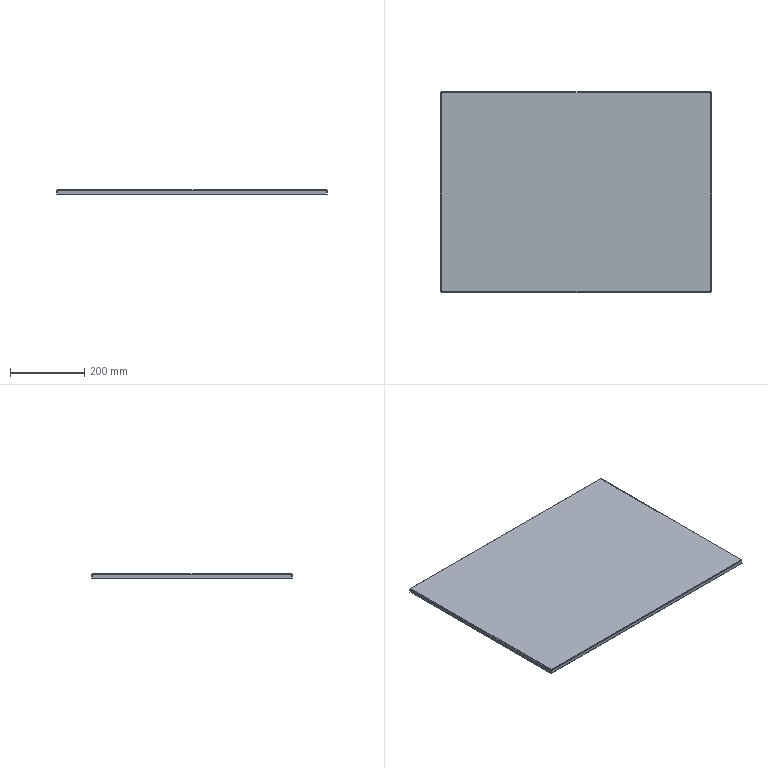Part | SolidWorks | features EdgeFlange 3, FlatPattern 1, SMBaseFlange 1, SMMiteredFlange 1, SheetMetal 1 | 1 solid | 42 faces | box 729.5 x 540 x 11.5 mm | volume 626320 mm3 | plane 34 | cylinder 8 | commonest cylinder face diameters 1.473 x4 4.473 x4
STEP:
#1=CARTESIAN_POINT('',(361.763,268.5,0.));
#2=VERTEX_POINT('',#1);
#3=CARTESIAN_POINT('',(361.763,268.5,-0.1248));
#4=VERTEX_POINT('',#3);
#5=CARTESIAN_POINT('',(361.763,268.5,0.));
#6=DIRECTION('',(0.,0.,-1.));
#7=VECTOR('',#6,1000.);
#8=LINE('',#5,#7);
#9=EDGE_CURVE('',#2,#4,#8,.T.);
#10=ORIENTED_EDGE('',*,*,#9,.T.);
#11=CARTESIAN_POINT('',(361.763,267.763,0.));
#12=VERTEX_POINT('',#11);
#13=CARTESIAN_POINT('',(361.763,267.763,-2.237));
#14=DIRECTION('',(1.,0.,0.));
#15=DIRECTION('',(0.,0.,-1.));
#16=AXIS2_PLACEMENT_3D('',#13,#14,#15);
#17=CIRCLE('',#16,2.237);
#18=EDGE_CURVE('',#4,#12,#17,.T.);
#19=ORIENTED_EDGE('',*,*,#18,.T.);
#20=CARTESIAN_POINT('',(361.763,-2953.5,0.));
#21=DIRECTION('',(0.,1.,0.));
#22=VECTOR('',#21,1000.);
#23=LINE('',#20,#22);
#24=EDGE_CURVE('',#12,#2,#23,.T.);
#25=ORIENTED_EDGE('',*,*,#24,.T.);
#26=EDGE_LOOP('',(#10,#19,#25));
#27=FACE_OUTER_BOUND('',#26,.T.);
#28=CARTESIAN_POINT('',(361.763,268.5,-1.5));
#29=DIRECTION('',(-1.,0.,0.));
#30=DIRECTION('',(0.,-1.,0.));
#31=AXIS2_PLACEMENT_3D('',#28,#29,#30);
#32=PLANE('',#31);
#33=ADVANCED_FACE('',(#27),#32,.T.);
#34=CARTESIAN_POINT('',(-363.263,268.5,0.));
#35=VERTEX_POINT('',#34);
#36=CARTESIAN_POINT('',(-363.263,267.763,0.));
#37=VERTEX_POINT('',#36);
#38=CARTESIAN_POINT('',(-363.263,268.5,0.));
#39=DIRECTION('',(0.,-1.,0.));
#40=VECTOR('',#39,1000.);
#41=LINE('',#38,#40);
#42=EDGE_CURVE('',#35,#37,#41,.T.);
#43=ORIENTED_EDGE('',*,*,#42,.T.);
#44=CARTESIAN_POINT('',(-363.263,268.5,-0.1248));
#45=VERTEX_POINT('',#44);
#46=CARTESIAN_POINT('',(-363.263,267.763,-2.237));
#47=DIRECTION('',(-1.,0.,0.));
#48=DIRECTION('',(0.,0.,-1.));
#49=AXIS2_PLACEMENT_3D('',#46,#47,#48);
#50=CIRCLE('',#49,2.237);
#51=EDGE_CURVE('',#37,#45,#50,.T.);
#52=ORIENTED_EDGE('',*,*,#51,.T.);
#53=CARTESIAN_POINT('',(-363.263,268.5,-1.5));
#54=DIRECTION('',(0.,0.,1.));
#55=VECTOR('',#54,1000.);
#56=LINE('',#53,#55);
#57=EDGE_CURVE('',#45,#35,#56,.T.);
#58=ORIENTED_EDGE('',*,*,#57,.T.);
#59=EDGE_LOOP('',(#43,#52,#58));
#60=FACE_OUTER_BOUND('',#59,.T.);
#61=CARTESIAN_POINT('',(-363.263,267.763,-1.5));
#62=DIRECTION('',(1.,0.,0.));
#63=DIRECTION('',(0.,0.,-1.));
#64=AXIS2_PLACEMENT_3D('',#61,#62,#63);
#65=PLANE('',#64);
#66=ADVANCED_FACE('',(#60),#65,.T.);
#67=CARTESIAN_POINT('',(361.763,267.763,-1.5));
#68=VERTEX_POINT('',#67);
#69=CARTESIAN_POINT('',(-363.263,267.763,-1.5));
#70=VERTEX_POINT('',#69);
#71=CARTESIAN_POINT('',(361.763,267.763,-1.5));
#72=DIRECTION('',(-1.,0.,0.));
#73=VECTOR('',#72,1000.);
#74=LINE('',#71,#73);
#75=EDGE_CURVE('',#68,#70,#74,.T.);
#76=ORIENTED_EDGE('',*,*,#75,.F.);
#77=CARTESIAN_POINT('',(361.763,-267.763,-1.5));
#78=VERTEX_POINT('',#77);
#79=CARTESIAN_POINT('',(361.763,-2953.5,-1.5));
#80=DIRECTION('',(0.,1.,0.));
#81=VECTOR('',#80,1000.);
#82=LINE('',#79,#81);
#83=EDGE_CURVE('',#78,#68,#82,.T.);
#84=ORIENTED_EDGE('',*,*,#83,.F.);
#85=CARTESIAN_POINT('',(-363.263,-267.763,-1.5));
#86=VERTEX_POINT('',#85);
#87=CARTESIAN_POINT('',(-364.,-267.763,-1.5));
#88=DIRECTION('',(1.,0.,0.));
#89=VECTOR('',#88,1000.);
#90=LINE('',#87,#89);
#91=EDGE_CURVE('',#86,#78,#90,.T.);
#92=ORIENTED_EDGE('',*,*,#91,.F.);
#93=CARTESIAN_POINT('',(-363.263,268.5,-1.5));
#94=DIRECTION('',(0.,-1.,0.));
#95=VECTOR('',#94,1000.);
#96=LINE('',#93,#95);
#97=EDGE_CURVE('',#70,#86,#96,.T.);
#98=ORIENTED_EDGE('',*,*,#97,.F.);
#99=EDGE_LOOP('',(#76,#84,#92,#98));
#100=FACE_OUTER_BOUND('',#99,.T.);
#101=CARTESIAN_POINT('',(0.,0.,-1.5));
#102=DIRECTION('',(0.,0.,1.));
#103=DIRECTION('',(1.,0.,0.));
#104=AXIS2_PLACEMENT_3D('',#101,#102,#103);
#105=PLANE('',#104);
#106=ADVANCED_FACE('',(#100),#105,.F.);
#107=CARTESIAN_POINT('',(361.763,-267.763,0.));
#108=VERTEX_POINT('',#107);
#109=CARTESIAN_POINT('',(361.763,-2953.5,0.));
#110=DIRECTION('',(0.,1.,0.));
#111=VECTOR('',#110,1000.);
#112=LINE('',#109,#111);
#113=EDGE_CURVE('',#108,#12,#112,.T.);
#114=ORIENTED_EDGE('',*,*,#113,.T.);
#115=CARTESIAN_POINT('',(361.763,267.763,0.));
#116=DIRECTION('',(-1.,0.,0.));
#117=VECTOR('',#116,1000.);
#118=LINE('',#115,#117);
#119=EDGE_CURVE('',#12,#37,#118,.T.);
#120=ORIENTED_EDGE('',*,*,#119,.T.);
#121=CARTESIAN_POINT('',(-363.263,-267.763,0.));
#122=VERTEX_POINT('',#121);
#123=CARTESIAN_POINT('',(-363.263,268.5,0.));
#124=DIRECTION('',(0.,-1.,0.));
#125=VECTOR('',#124,1000.);
#126=LINE('',#123,#125);
#127=EDGE_CURVE('',#37,#122,#126,.T.);
#128=ORIENTED_EDGE('',*,*,#127,.T.);
#129=CARTESIAN_POINT('',(-364.,-267.763,0.));
#130=DIRECTION('',(1.,0.,0.));
#131=VECTOR('',#130,1000.);
#132=LINE('',#129,#131);
#133=EDGE_CURVE('',#122,#108,#132,.T.);
#134=ORIENTED_EDGE('',*,*,#133,.T.);
#135=EDGE_LOOP('',(#114,#120,#128,#134));
#136=FACE_OUTER_BOUND('',#135,.T.);
#137=CARTESIAN_POINT('',(0.,0.,0.));
#138=DIRECTION('',(0.,0.,1.));
#139=DIRECTION('',(1.,0.,0.));
#140=AXIS2_PLACEMENT_3D('',#137,#138,#139);
#141=PLANE('',#140);
#142=ADVANCED_FACE('',(#136),#141,.T.);
#143=CARTESIAN_POINT('',(-364.,-267.763,0.));
#144=VERTEX_POINT('',#143);
#145=CARTESIAN_POINT('',(-364.,-267.763,0.));
#146=DIRECTION('',(1.,0.,0.));
#147=VECTOR('',#146,1000.);
#148=LINE('',#145,#147);
#149=EDGE_CURVE('',#144,#122,#148,.T.);
#150=ORIENTED_EDGE('',*,*,#149,.T.);
#151=CARTESIAN_POINT('',(-364.,-267.763,-0.1248));
#152=VERTEX_POINT('',#151);
#153=CARTESIAN_POINT('',(-363.263,-267.763,-2.237));
#154=DIRECTION('',(0.,-1.,0.));
#155=DIRECTION('',(0.,0.,1.));
#156=AXIS2_PLACEMENT_3D('',#153,#154,#155);
#157=CIRCLE('',#156,2.237);
#158=EDGE_CURVE('',#122,#152,#157,.T.);
#159=ORIENTED_EDGE('',*,*,#158,.T.);
#160=CARTESIAN_POINT('',(-364.,-267.763,-1.5));
#161=DIRECTION('',(0.,0.,1.));
#162=VECTOR('',#161,1000.);
#163=LINE('',#160,#162);
#164=EDGE_CURVE('',#152,#144,#163,.T.);
#165=ORIENTED_EDGE('',*,*,#164,.T.);
#166=EDGE_LOOP('',(#150,#159,#165));
#167=FACE_OUTER_BOUND('',#166,.T.);
#168=CARTESIAN_POINT('',(-363.263,-267.763,-1.5));
#169=DIRECTION('',(0.,1.,0.));
#170=DIRECTION('',(-1.,0.,0.));
#171=AXIS2_PLACEMENT_3D('',#168,#169,#170);
#172=PLANE('',#171);
#173=ADVANCED_FACE('',(#167),#172,.T.);
#174=CARTESIAN_POINT('',(361.763,-268.5,0.));
#175=VERTEX_POINT('',#174);
#176=CARTESIAN_POINT('',(361.763,-2953.5,0.));
#177=DIRECTION('',(0.,1.,0.));
#178=VECTOR('',#177,1000.);
#179=LINE('',#176,#178);
#180=EDGE_CURVE('',#175,#108,#179,.T.);
#181=ORIENTED_EDGE('',*,*,#180,.T.);
#182=CARTESIAN_POINT('',(361.763,-268.5,-0.1248));
#183=VERTEX_POINT('',#182);
#184=CARTESIAN_POINT('',(361.763,-267.763,-2.237));
#185=DIRECTION('',(1.,0.,0.));
#186=DIRECTION('',(0.,0.,1.));
#187=AXIS2_PLACEMENT_3D('',#184,#185,#186);
#188=CIRCLE('',#187,2.237);
#189=EDGE_CURVE('',#108,#183,#188,.T.);
#190=ORIENTED_EDGE('',*,*,#189,.T.);
#191=CARTESIAN_POINT('',(361.763,-268.5,0.));
#192=DIRECTION('',(0.,0.,-1.));
#193=VECTOR('',#192,1000.);
#194=LINE('',#191,#193);
#195=EDGE_CURVE('',#175,#183,#194,.T.);
#196=ORIENTED_EDGE('',*,*,#195,.F.);
#197=EDGE_LOOP('',(#181,#190,#196));
#198=FACE_OUTER_BOUND('',#197,.T.);
#199=CARTESIAN_POINT('',(361.763,-267.763,-1.5));
#200=DIRECTION('',(-1.,0.,0.));
#201=DIRECTION('',(0.,0.,1.));
#202=AXIS2_PLACEMENT_3D('',#199,#200,#201);
#203=PLANE('',#202);
#204=ADVANCED_FACE('',(#198),#203,.T.);
#205=CARTESIAN_POINT('',(364.,268.5,-11.5));
#206=VERTEX_POINT('',#205);
#207=CARTESIAN_POINT('',(362.5,268.5,-11.5));
#208=VERTEX_POINT('',#207);
#209=CARTESIAN_POINT('',(364.,268.5,-11.5));
#210=DIRECTION('',(-1.,0.,0.));
#211=VECTOR('',#210,1000.);
#212=LINE('',#209,#211);
#213=EDGE_CURVE('',#206,#208,#212,.T.);
#214=ORIENTED_EDGE('',*,*,#213,.F.);
#215=CARTESIAN_POINT('',(364.,-268.5,-11.5));
#216=VERTEX_POINT('',#215);
#217=CARTESIAN_POINT('',(364.,-268.5,-11.5));
#218=DIRECTION('',(0.,1.,0.));
#219=VECTOR('',#218,1000.);
#220=LINE('',#217,#219);
#221=EDGE_CURVE('',#216,#206,#220,.T.);
#222=ORIENTED_EDGE('',*,*,#221,.F.);
#223=CARTESIAN_POINT('',(362.5,-268.5,-11.5));
#224=VERTEX_POINT('',#223);
#225=CARTESIAN_POINT('',(364.,-268.5,-11.5));
#226=DIRECTION('',(-1.,0.,0.));
#227=VECTOR('',#226,1000.);
#228=LINE('',#225,#227);
#229=EDGE_CURVE('',#216,#224,#228,.T.);
#230=ORIENTED_EDGE('',*,*,#229,.T.);
#231=CARTESIAN_POINT('',(362.5,-268.5,-11.5));
#232=DIRECTION('',(0.,1.,0.));
#233=VECTOR('',#232,1000.);
#234=LINE('',#231,#233);
#235=EDGE_CURVE('',#224,#208,#234,.T.);
#236=ORIENTED_EDGE('',*,*,#235,.T.);
#237=EDGE_LOOP('',(#214,#222,#230,#236));
#238=FACE_OUTER_BOUND('',#237,.T.);
#239=CARTESIAN_POINT('',(364.,-268.5,-11.5));
#240=DIRECTION('',(0.,0.,1.));
#241=DIRECTION('',(0.,1.,0.));
#242=AXIS2_PLACEMENT_3D('',#239,#240,#241);
#243=PLANE('',#242);
#244=ADVANCED_FACE('',(#238),#243,.F.);
#245=ORIENTED_EDGE('',*,*,#229,.F.);
#246=CARTESIAN_POINT('',(364.,-268.5,-2.237));
#247=VERTEX_POINT('',#246);
#248=CARTESIAN_POINT('',(364.,-268.5,-11.5));
#249=DIRECTION('',(0.,0.,1.));
#250=VECTOR('',#249,1000.);
#251=LINE('',#248,#250);
#252=EDGE_CURVE('',#216,#247,#251,.T.);
#253=ORIENTED_EDGE('',*,*,#252,.T.);
#254=CARTESIAN_POINT('',(362.5,-268.5,-2.237));
#255=VERTEX_POINT('',#254);
#256=CARTESIAN_POINT('',(364.,-268.5,-2.237));
#257=DIRECTION('',(-1.,0.,0.));
#258=VECTOR('',#257,1000.);
#259=LINE('',#256,#258);
#260=EDGE_CURVE('',#247,#255,#259,.T.);
#261=ORIENTED_EDGE('',*,*,#260,.T.);
#262=CARTESIAN_POINT('',(362.5,-268.5,-11.5));
#263=DIRECTION('',(0.,0.,1.));
#264=VECTOR('',#263,1000.);
#265=LINE('',#262,#264);
#266=EDGE_CURVE('',#224,#255,#265,.T.);
#267=ORIENTED_EDGE('',*,*,#266,.F.);
#268=EDGE_LOOP('',(#245,#253,#261,#267));
#269=FACE_OUTER_BOUND('',#268,.T.);
#270=CARTESIAN_POINT('',(364.,-268.5,-11.5));
#271=DIRECTION('',(0.,-1.,0.));
#272=DIRECTION('',(0.,0.,1.));
#273=AXIS2_PLACEMENT_3D('',#270,#271,#272);
#274=PLANE('',#273);
#275=ADVANCED_FACE('',(#269),#274,.T.);
#276=CARTESIAN_POINT('',(364.,268.5,-2.237));
#277=VERTEX_POINT('',#276);
#278=CARTESIAN_POINT('',(364.,268.5,-11.5));
#279=DIRECTION('',(0.,0.,-1.));
#280=VECTOR('',#279,1000.);
#281=LINE('',#278,#280);
#282=EDGE_CURVE('',#277,#206,#281,.T.);
#283=ORIENTED_EDGE('',*,*,#282,.T.);
#284=ORIENTED_EDGE('',*,*,#213,.T.);
#285=CARTESIAN_POINT('',(362.5,268.5,-2.237));
#286=VERTEX_POINT('',#285);
#287=CARTESIAN_POINT('',(362.5,268.5,-11.5));
#288=DIRECTION('',(0.,0.,-1.));
#289=VECTOR('',#288,1000.);
#290=LINE('',#287,#289);
#291=EDGE_CURVE('',#286,#208,#290,.T.);
#292=ORIENTED_EDGE('',*,*,#291,.F.);
#293=CARTESIAN_POINT('',(364.,268.5,-2.237));
#294=DIRECTION('',(-1.,0.,0.));
#295=VECTOR('',#294,1000.);
#296=LINE('',#293,#295);
#297=EDGE_CURVE('',#277,#286,#296,.T.);
#298=ORIENTED_EDGE('',*,*,#297,.F.);
#299=EDGE_LOOP('',(#283,#284,#292,#298));
#300=FACE_OUTER_BOUND('',#299,.T.);
#301=CARTESIAN_POINT('',(364.,268.5,-11.5));
#302=DIRECTION('',(0.,1.,0.));
#303=DIRECTION('',(0.,0.,-1.));
#304=AXIS2_PLACEMENT_3D('',#301,#302,#303);
#305=PLANE('',#304);
#306=ADVANCED_FACE('',(#300),#305,.T.);
#307=CARTESIAN_POINT('',(362.5,-268.5,-2.237));
#308=DIRECTION('',(0.,1.,0.));
#309=VECTOR('',#308,1000.);
#310=LINE('',#307,#309);
#311=EDGE_CURVE('',#255,#286,#310,.T.);
#312=ORIENTED_EDGE('',*,*,#311,.T.);
#313=ORIENTED_EDGE('',*,*,#291,.T.);
#314=ORIENTED_EDGE('',*,*,#235,.F.);
#315=ORIENTED_EDGE('',*,*,#266,.T.);
#316=EDGE_LOOP('',(#312,#313,#314,#315));
#317=FACE_OUTER_BOUND('',#316,.T.);
#318=CARTESIAN_POINT('',(362.5,-268.5,-11.5));
#319=DIRECTION('',(-1.,0.,0.));
#320=DIRECTION('',(0.,0.,1.));
#321=AXIS2_PLACEMENT_3D('',#318,#319,#320);
#322=PLANE('',#321);
#323=ADVANCED_FACE('',(#317),#322,.T.);
#324=CARTESIAN_POINT('',(364.,-268.5,-2.237));
#325=DIRECTION('',(0.,1.,0.));
#326=VECTOR('',#325,1000.);
#327=LINE('',#324,#326);
#328=EDGE_CURVE('',#247,#277,#327,.T.);
#329=ORIENTED_EDGE('',*,*,#328,.F.);
#330=ORIENTED_EDGE('',*,*,#252,.F.);
#331=ORIENTED_EDGE('',*,*,#221,.T.);
#332=ORIENTED_EDGE('',*,*,#282,.F.);
#333=EDGE_LOOP('',(#329,#330,#331,#332));
#334=FACE_OUTER_BOUND('',#333,.T.);
#335=CARTESIAN_POINT('',(364.,-268.5,-11.5));
#336=DIRECTION('',(-1.,0.,0.));
#337=DIRECTION('',(0.,0.,1.));
#338=AXIS2_PLACEMENT_3D('',#335,#336,#337);
#339=PLANE('',#338);
#340=ADVANCED_FACE('',(#334),#339,.F.);
#341=ORIENTED_EDGE('',*,*,#260,.F.);
#342=CARTESIAN_POINT('',(361.763,-268.5,-2.237));
#343=DIRECTION('',(0.,-1.,0.));
#344=DIRECTION('',(1.,0.,0.));
#345=AXIS2_PLACEMENT_3D('',#342,#343,#344);
#346=CIRCLE('',#345,2.237);
#347=EDGE_CURVE('',#247,#175,#346,.T.);
#348=ORIENTED_EDGE('',*,*,#347,.T.);
#349=ORIENTED_EDGE('',*,*,#195,.T.);
#350=CARTESIAN_POINT('',(361.763,-268.5,-1.5));
#351=VERTEX_POINT('',#350);
#352=CARTESIAN_POINT('',(361.763,-268.5,0.));
#353=DIRECTION('',(0.,0.,-1.));
#354=VECTOR('',#353,1000.);
#355=LINE('',#352,#354);
#356=EDGE_CURVE('',#183,#351,#355,.T.);
#357=ORIENTED_EDGE('',*,*,#356,.T.);
#358=CARTESIAN_POINT('',(361.763,-268.5,-2.237));
#359=DIRECTION('',(0.,-1.,0.));
#360=DIRECTION('',(-1.,0.,0.));
#361=AXIS2_PLACEMENT_3D('',#358,#359,#360);
#362=CIRCLE('',#361,0.7366);
#363=EDGE_CURVE('',#255,#351,#362,.T.);
#364=ORIENTED_EDGE('',*,*,#363,.F.);
#365=EDGE_LOOP('',(#341,#348,#349,#357,#364));
#366=FACE_OUTER_BOUND('',#365,.T.);
#367=CARTESIAN_POINT('',(361.763,-268.5,-2.237));
#368=DIRECTION('',(0.,1.,0.));
#369=DIRECTION('',(-1.,0.,0.));
#370=AXIS2_PLACEMENT_3D('',#367,#368,#369);
#371=PLANE('',#370);
#372=ADVANCED_FACE('',(#366),#371,.F.);
#373=CARTESIAN_POINT('',(361.763,268.5,-2.237));
#374=DIRECTION('',(0.,1.,0.));
#375=DIRECTION('',(-1.,0.,0.));
#376=AXIS2_PLACEMENT_3D('',#373,#374,#375);
#377=CIRCLE('',#376,2.237);
#378=EDGE_CURVE('',#2,#277,#377,.T.);
#379=ORIENTED_EDGE('',*,*,#378,.T.);
#380=ORIENTED_EDGE('',*,*,#297,.T.);
#381=CARTESIAN_POINT('',(361.763,268.5,-1.5));
#382=VERTEX_POINT('',#381);
#383=CARTESIAN_POINT('',(361.763,268.5,-2.237));
#384=DIRECTION('',(0.,1.,0.));
#385=DIRECTION('',(-1.,0.,0.));
#386=AXIS2_PLACEMENT_3D('',#383,#384,#385);
#387=CIRCLE('',#386,0.7366);
#388=EDGE_CURVE('',#382,#286,#387,.T.);
#389=ORIENTED_EDGE('',*,*,#388,.F.);
#390=CARTESIAN_POINT('',(361.763,268.5,0.));
#391=DIRECTION('',(0.,0.,-1.));
#392=VECTOR('',#391,1000.);
#393=LINE('',#390,#392);
#394=EDGE_CURVE('',#4,#382,#393,.T.);
#395=ORIENTED_EDGE('',*,*,#394,.F.);
#396=ORIENTED_EDGE('',*,*,#9,.F.);
#397=EDGE_LOOP('',(#379,#380,#389,#395,#396));
#398=FACE_OUTER_BOUND('',#397,.T.);
#399=CARTESIAN_POINT('',(361.763,268.5,-2.237));
#400=DIRECTION('',(0.,-1.,0.));
#401=DIRECTION('',(1.,0.,0.));
#402=AXIS2_PLACEMENT_3D('',#399,#400,#401);
#403=PLANE('',#402);
#404=ADVANCED_FACE('',(#398),#403,.F.);
#405=CARTESIAN_POINT('',(361.763,-2953.5,-1.5));
#406=DIRECTION('',(0.,1.,0.));
#407=VECTOR('',#406,1000.);
#408=LINE('',#405,#407);
#409=EDGE_CURVE('',#351,#78,#408,.T.);
#410=ORIENTED_EDGE('',*,*,#409,.T.);
#411=ORIENTED_EDGE('',*,*,#83,.T.);
#412=CARTESIAN_POINT('',(361.763,268.5,-1.5));
#413=DIRECTION('',(0.,-1.,0.));
#414=VECTOR('',#413,1000.);
#415=LINE('',#412,#414);
#416=EDGE_CURVE('',#382,#68,#415,.T.);
#417=ORIENTED_EDGE('',*,*,#416,.F.);
#418=ORIENTED_EDGE('',*,*,#388,.T.);
#419=ORIENTED_EDGE('',*,*,#311,.F.);
#420=ORIENTED_EDGE('',*,*,#363,.T.);
#421=EDGE_LOOP('',(#410,#411,#417,#418,#419,#420));
#422=FACE_OUTER_BOUND('',#421,.T.);
#423=CARTESIAN_POINT('',(361.763,-2953.5,-2.237));
#424=DIRECTION('',(0.,1.,0.));
#425=DIRECTION('',(-1.,0.,0.));
#426=AXIS2_PLACEMENT_3D('',#423,#424,#425);
#427=CYLINDRICAL_SURFACE('',#426,0.7366);
#428=ADVANCED_FACE('',(#422),#427,.F.);
#429=ORIENTED_EDGE('',*,*,#180,.F.);
#430=ORIENTED_EDGE('',*,*,#347,.F.);
#431=ORIENTED_EDGE('',*,*,#328,.T.);
#432=ORIENTED_EDGE('',*,*,#378,.F.);
#433=ORIENTED_EDGE('',*,*,#24,.F.);
#434=ORIENTED_EDGE('',*,*,#113,.F.);
#435=EDGE_LOOP('',(#429,#430,#431,#432,#433,#434));
#436=FACE_OUTER_BOUND('',#435,.T.);
#437=CARTESIAN_POINT('',(361.763,-2953.5,-2.237));
#438=DIRECTION('',(0.,1.,0.));
#439=DIRECTION('',(-1.,0.,0.));
#440=AXIS2_PLACEMENT_3D('',#437,#438,#439);
#441=CYLINDRICAL_SURFACE('',#440,2.237);
#442=ADVANCED_FACE('',(#436),#441,.T.);
#443=ORIENTED_EDGE('',*,*,#356,.F.);
#444=CARTESIAN_POINT('',(361.763,-270.,-2.237));
#445=VERTEX_POINT('',#444);
#446=CARTESIAN_POINT('',(361.763,-267.763,-2.237));
#447=DIRECTION('',(1.,0.,0.));
#448=DIRECTION('',(0.,0.,1.));
#449=AXIS2_PLACEMENT_3D('',#446,#447,#448);
#450=CIRCLE('',#449,2.237);
#451=EDGE_CURVE('',#183,#445,#450,.T.);
#452=ORIENTED_EDGE('',*,*,#451,.T.);
#453=CARTESIAN_POINT('',(361.763,-268.5,-2.237));
#454=VERTEX_POINT('',#453);
#455=CARTESIAN_POINT('',(361.763,-268.5,-2.237));
#456=DIRECTION('',(0.,-1.,0.));
#457=VECTOR('',#456,1000.);
#458=LINE('',#455,#457);
#459=EDGE_CURVE('',#454,#445,#458,.T.);
#460=ORIENTED_EDGE('',*,*,#459,.F.);
#461=CARTESIAN_POINT('',(361.763,-267.763,-2.237));
#462=DIRECTION('',(1.,0.,0.));
#463=DIRECTION('',(0.,0.,1.));
#464=AXIS2_PLACEMENT_3D('',#461,#462,#463);
#465=CIRCLE('',#464,0.7366);
#466=EDGE_CURVE('',#78,#454,#465,.T.);
#467=ORIENTED_EDGE('',*,*,#466,.F.);
#468=ORIENTED_EDGE('',*,*,#409,.F.);
#469=EDGE_LOOP('',(#443,#452,#460,#467,#468));
#470=FACE_OUTER_BOUND('',#469,.T.);
#471=CARTESIAN_POINT('',(361.763,-267.763,-2.237));
#472=DIRECTION('',(1.,0.,0.));
#473=DIRECTION('',(0.,0.,-1.));
#474=AXIS2_PLACEMENT_3D('',#471,#472,#473);
#475=PLANE('',#474);
#476=ADVANCED_FACE('',(#470),#475,.T.);
#477=CARTESIAN_POINT('',(-364.,-268.5,-2.237));
#478=VERTEX_POINT('',#477);
#479=CARTESIAN_POINT('',(-364.,-267.763,-1.5));
#480=VERTEX_POINT('',#479);
#481=CARTESIAN_POINT('',(-364.,-267.763,-2.237));
#482=DIRECTION('',(-1.,0.,0.));
#483=DIRECTION('',(0.,0.,1.));
#484=AXIS2_PLACEMENT_3D('',#481,#482,#483);
#485=CIRCLE('',#484,0.7366);
#486=EDGE_CURVE('',#478,#480,#485,.T.);
#487=ORIENTED_EDGE('',*,*,#486,.F.);
#488=CARTESIAN_POINT('',(-364.,-270.,-2.237));
#489=VERTEX_POINT('',#488);
#490=CARTESIAN_POINT('',(-364.,-268.5,-2.237));
#491=DIRECTION('',(0.,-1.,0.));
#492=VECTOR('',#491,1000.);
#493=LINE('',#490,#492);
#494=EDGE_CURVE('',#478,#489,#493,.T.);
#495=ORIENTED_EDGE('',*,*,#494,.T.);
#496=CARTESIAN_POINT('',(-364.,-267.763,-2.237));
#497=DIRECTION('',(-1.,0.,0.));
#498=DIRECTION('',(0.,0.,1.));
#499=AXIS2_PLACEMENT_3D('',#496,#497,#498);
#500=CIRCLE('',#499,2.237);
#501=EDGE_CURVE('',#489,#144,#500,.T.);
#502=ORIENTED_EDGE('',*,*,#501,.T.);
#503=ORIENTED_EDGE('',*,*,#164,.F.);
#504=CARTESIAN_POINT('',(-364.,-267.763,-1.5));
#505=DIRECTION('',(0.,0.,1.));
#506=VECTOR('',#505,1000.);
#507=LINE('',#504,#506);
#508=EDGE_CURVE('',#480,#152,#507,.T.);
#509=ORIENTED_EDGE('',*,*,#508,.F.);
#510=EDGE_LOOP('',(#487,#495,#502,#503,#509));
#511=FACE_OUTER_BOUND('',#510,.T.);
#512=CARTESIAN_POINT('',(-364.,-267.763,-2.237));
#513=DIRECTION('',(1.,0.,0.));
#514=DIRECTION('',(0.,0.,-1.));
#515=AXIS2_PLACEMENT_3D('',#512,#513,#514);
#516=PLANE('',#515);
#517=ADVANCED_FACE('',(#511),#516,.F.);
#518=ORIENTED_EDGE('',*,*,#149,.F.);
#519=ORIENTED_EDGE('',*,*,#501,.F.);
#520=CARTESIAN_POINT('',(0.,-270.,-2.237));
#521=DIRECTION('',(1.,0.,0.));
#522=VECTOR('',#521,1000.);
#523=LINE('',#520,#522);
#524=EDGE_CURVE('',#489,#445,#523,.T.);
#525=ORIENTED_EDGE('',*,*,#524,.T.);
#526=ORIENTED_EDGE('',*,*,#451,.F.);
#527=ORIENTED_EDGE('',*,*,#189,.F.);
#528=ORIENTED_EDGE('',*,*,#133,.F.);
#529=EDGE_LOOP('',(#518,#519,#525,#526,#527,#528));
#530=FACE_OUTER_BOUND('',#529,.T.);
#531=CARTESIAN_POINT('',(-364.,-267.763,-2.237));
#532=DIRECTION('',(-1.,0.,0.));
#533=DIRECTION('',(0.,-1.,0.));
#534=AXIS2_PLACEMENT_3D('',#531,#532,#533);
#535=CYLINDRICAL_SURFACE('',#534,2.237);
#536=ADVANCED_FACE('',(#530),#535,.T.);
#537=CARTESIAN_POINT('',(-364.,-267.763,-1.5));
#538=DIRECTION('',(1.,0.,0.));
#539=VECTOR('',#538,1000.);
#540=LINE('',#537,#539);
#541=EDGE_CURVE('',#480,#86,#540,.T.);
#542=ORIENTED_EDGE('',*,*,#541,.T.);
#543=ORIENTED_EDGE('',*,*,#91,.T.);
#544=ORIENTED_EDGE('',*,*,#466,.T.);
#545=CARTESIAN_POINT('',(361.763,-268.5,-2.237));
#546=DIRECTION('',(-1.,0.,0.));
#547=VECTOR('',#546,1000.);
#548=LINE('',#545,#547);
#549=EDGE_CURVE('',#454,#478,#548,.T.);
#550=ORIENTED_EDGE('',*,*,#549,.T.);
#551=ORIENTED_EDGE('',*,*,#486,.T.);
#552=EDGE_LOOP('',(#542,#543,#544,#550,#551));
#553=FACE_OUTER_BOUND('',#552,.T.);
#554=CARTESIAN_POINT('',(-364.,-267.763,-2.237));
#555=DIRECTION('',(-1.,0.,0.));
#556=DIRECTION('',(0.,-1.,0.));
#557=AXIS2_PLACEMENT_3D('',#554,#555,#556);
#558=CYLINDRICAL_SURFACE('',#557,0.7366);
#559=ADVANCED_FACE('',(#553),#558,.F.);
#560=ORIENTED_EDGE('',*,*,#494,.F.);
#561=CARTESIAN_POINT('',(-364.,-268.5,-11.5));
#562=VERTEX_POINT('',#561);
#563=CARTESIAN_POINT('',(-364.,-268.5,-11.5));
#564=DIRECTION('',(0.,0.,-1.));
#565=VECTOR('',#564,1000.);
#566=LINE('',#563,#565);
#567=EDGE_CURVE('',#478,#562,#566,.T.);
#568=ORIENTED_EDGE('',*,*,#567,.T.);
#569=CARTESIAN_POINT('',(-364.,-270.,-11.5));
#570=VERTEX_POINT('',#569);
#571=CARTESIAN_POINT('',(-364.,-270.,-11.5));
#572=DIRECTION('',(0.,1.,0.));
#573=VECTOR('',#572,1000.);
#574=LINE('',#571,#573);
#575=EDGE_CURVE('',#570,#562,#574,.T.);
#576=ORIENTED_EDGE('',*,*,#575,.F.);
#577=CARTESIAN_POINT('',(-364.,-270.,-11.5));
#578=DIRECTION('',(0.,0.,-1.));
#579=VECTOR('',#578,1000.);
#580=LINE('',#577,#579);
#581=EDGE_CURVE('',#489,#570,#580,.T.);
#582=ORIENTED_EDGE('',*,*,#581,.F.);
#583=EDGE_LOOP('',(#560,#568,#576,#582));
#584=FACE_OUTER_BOUND('',#583,.T.);
#585=CARTESIAN_POINT('',(-364.,-270.,-11.5));
#586=DIRECTION('',(1.,0.,0.));
#587=DIRECTION('',(0.,0.,-1.));
#588=AXIS2_PLACEMENT_3D('',#585,#586,#587);
#589=PLANE('',#588);
#590=ADVANCED_FACE('',(#584),#589,.F.);
#591=ORIENTED_EDGE('',*,*,#459,.T.);
#592=CARTESIAN_POINT('',(361.763,-270.,-11.5));
#593=VERTEX_POINT('',#592);
#594=CARTESIAN_POINT('',(361.763,-270.,-1.5));
#595=DIRECTION('',(0.,0.,1.));
#596=VECTOR('',#595,1000.);
#597=LINE('',#594,#596);
#598=EDGE_CURVE('',#593,#445,#597,.T.);
#599=ORIENTED_EDGE('',*,*,#598,.F.);
#600=CARTESIAN_POINT('',(361.763,-268.5,-11.5));
#601=VERTEX_POINT('',#600);
#602=CARTESIAN_POINT('',(361.763,-270.,-11.5));
#603=DIRECTION('',(0.,1.,0.));
#604=VECTOR('',#603,1000.);
#605=LINE('',#602,#604);
#606=EDGE_CURVE('',#593,#601,#605,.T.);
#607=ORIENTED_EDGE('',*,*,#606,.T.);
#608=CARTESIAN_POINT('',(361.763,-268.5,-1.5));
#609=DIRECTION('',(0.,0.,1.));
#610=VECTOR('',#609,1000.);
#611=LINE('',#608,#610);
#612=EDGE_CURVE('',#601,#454,#611,.T.);
#613=ORIENTED_EDGE('',*,*,#612,.T.);
#614=EDGE_LOOP('',(#591,#599,#607,#613));
#615=FACE_OUTER_BOUND('',#614,.T.);
#616=CARTESIAN_POINT('',(361.763,-270.,-1.5));
#617=DIRECTION('',(-1.,0.,0.));
#618=DIRECTION('',(0.,0.,1.));
#619=AXIS2_PLACEMENT_3D('',#616,#617,#618);
#620=PLANE('',#619);
#621=ADVANCED_FACE('',(#615),#620,.F.);
#622=ORIENTED_EDGE('',*,*,#524,.F.);
#623=ORIENTED_EDGE('',*,*,#581,.T.);
#624=CARTESIAN_POINT('',(361.763,-270.,-11.5));
#625=DIRECTION('',(1.,0.,0.));
#626=VECTOR('',#625,1000.);
#627=LINE('',#624,#626);
#628=EDGE_CURVE('',#570,#593,#627,.T.);
#629=ORIENTED_EDGE('',*,*,#628,.T.);
#630=ORIENTED_EDGE('',*,*,#598,.T.);
#631=EDGE_LOOP('',(#622,#623,#629,#630));
#632=FACE_OUTER_BOUND('',#631,.T.);
#633=CARTESIAN_POINT('',(0.,-270.,0.));
#634=DIRECTION('',(0.,1.,0.));
#635=DIRECTION('',(0.,0.,1.));
#636=AXIS2_PLACEMENT_3D('',#633,#634,#635);
#637=PLANE('',#636);
#638=ADVANCED_FACE('',(#632),#637,.F.);
#639=ORIENTED_EDGE('',*,*,#567,.F.);
#640=ORIENTED_EDGE('',*,*,#549,.F.);
#641=ORIENTED_EDGE('',*,*,#612,.F.);
#642=CARTESIAN_POINT('',(361.763,-268.5,-11.5));
#643=DIRECTION('',(1.,0.,0.));
#644=VECTOR('',#643,1000.);
#645=LINE('',#642,#644);
#646=EDGE_CURVE('',#562,#601,#645,.T.);
#647=ORIENTED_EDGE('',*,*,#646,.F.);
#648=EDGE_LOOP('',(#639,#640,#641,#647));
#649=FACE_OUTER_BOUND('',#648,.T.);
#650=CARTESIAN_POINT('',(0.,-268.5,0.));
#651=DIRECTION('',(0.,1.,0.));
#652=DIRECTION('',(0.,0.,1.));
#653=AXIS2_PLACEMENT_3D('',#650,#651,#652);
#654=PLANE('',#653);
#655=ADVANCED_FACE('',(#649),#654,.T.);
#656=ORIENTED_EDGE('',*,*,#646,.T.);
#657=ORIENTED_EDGE('',*,*,#606,.F.);
#658=ORIENTED_EDGE('',*,*,#628,.F.);
#659=ORIENTED_EDGE('',*,*,#575,.T.);
#660=EDGE_LOOP('',(#656,#657,#658,#659));
#661=FACE_OUTER_BOUND('',#660,.T.);
#662=CARTESIAN_POINT('',(361.763,-270.,-11.5));
#663=DIRECTION('',(0.,0.,1.));
#664=DIRECTION('',(0.,-1.,0.));
#665=AXIS2_PLACEMENT_3D('',#662,#663,#664);
#666=PLANE('',#665);
#667=ADVANCED_FACE('',(#661),#666,.F.);
#668=ORIENTED_EDGE('',*,*,#541,.F.);
#669=ORIENTED_EDGE('',*,*,#508,.T.);
#670=CARTESIAN_POINT('',(-365.5,-267.763,-2.237));
#671=VERTEX_POINT('',#670);
#672=CARTESIAN_POINT('',(-363.263,-267.763,-2.237));
#673=DIRECTION('',(0.,-1.,0.));
#674=DIRECTION('',(0.,0.,1.));
#675=AXIS2_PLACEMENT_3D('',#672,#673,#674);
#676=CIRCLE('',#675,2.237);
#677=EDGE_CURVE('',#152,#671,#676,.T.);
#678=ORIENTED_EDGE('',*,*,#677,.T.);
#679=CARTESIAN_POINT('',(-364.,-267.763,-2.237));
#680=VERTEX_POINT('',#679);
#681=CARTESIAN_POINT('',(-364.,-267.763,-2.237));
#682=DIRECTION('',(-1.,0.,0.));
#683=VECTOR('',#682,1000.);
#684=LINE('',#681,#683);
#685=EDGE_CURVE('',#680,#671,#684,.T.);
#686=ORIENTED_EDGE('',*,*,#685,.F.);
#687=CARTESIAN_POINT('',(-363.263,-267.763,-2.237));
#688=DIRECTION('',(0.,-1.,0.));
#689=DIRECTION('',(0.,0.,1.));
#690=AXIS2_PLACEMENT_3D('',#687,#688,#689);
#691=CIRCLE('',#690,0.7366);
#692=EDGE_CURVE('',#86,#680,#691,.T.);
#693=ORIENTED_EDGE('',*,*,#692,.F.);
#694=EDGE_LOOP('',(#668,#669,#678,#686,#693));
#695=FACE_OUTER_BOUND('',#694,.T.);
#696=CARTESIAN_POINT('',(-363.263,-267.763,-2.237));
#697=DIRECTION('',(0.,-1.,0.));
#698=DIRECTION('',(0.,0.,-1.));
#699=AXIS2_PLACEMENT_3D('',#696,#697,#698);
#700=PLANE('',#699);
#701=ADVANCED_FACE('',(#695),#700,.T.);
#702=CARTESIAN_POINT('',(-364.,268.5,-2.237));
#703=VERTEX_POINT('',#702);
#704=CARTESIAN_POINT('',(-363.263,268.5,-1.5));
#705=VERTEX_POINT('',#704);
#706=CARTESIAN_POINT('',(-363.263,268.5,-2.237));
#707=DIRECTION('',(0.,1.,0.));
#708=DIRECTION('',(0.,0.,1.));
#709=AXIS2_PLACEMENT_3D('',#706,#707,#708);
#710=CIRCLE('',#709,0.7366);
#711=EDGE_CURVE('',#703,#705,#710,.T.);
#712=ORIENTED_EDGE('',*,*,#711,.F.);
#713=CARTESIAN_POINT('',(-365.5,268.5,-2.237));
#714=VERTEX_POINT('',#713);
#715=CARTESIAN_POINT('',(-364.,268.5,-2.237));
#716=DIRECTION('',(-1.,0.,0.));
#717=VECTOR('',#716,1000.);
#718=LINE('',#715,#717);
#719=EDGE_CURVE('',#703,#714,#718,.T.);
#720=ORIENTED_EDGE('',*,*,#719,.T.);
#721=CARTESIAN_POINT('',(-363.263,268.5,-2.237));
#722=DIRECTION('',(0.,1.,0.));
#723=DIRECTION('',(0.,0.,1.));
#724=AXIS2_PLACEMENT_3D('',#721,#722,#723);
#725=CIRCLE('',#724,2.237);
#726=EDGE_CURVE('',#714,#35,#725,.T.);
#727=ORIENTED_EDGE('',*,*,#726,.T.);
#728=ORIENTED_EDGE('',*,*,#57,.F.);
#729=CARTESIAN_POINT('',(-363.263,268.5,-1.5));
#730=DIRECTION('',(0.,0.,1.));
#731=VECTOR('',#730,1000.);
#732=LINE('',#729,#731);
#733=EDGE_CURVE('',#705,#45,#732,.T.);
#734=ORIENTED_EDGE('',*,*,#733,.F.);
#735=EDGE_LOOP('',(#712,#720,#727,#728,#734));
#736=FACE_OUTER_BOUND('',#735,.T.);
#737=CARTESIAN_POINT('',(-363.263,268.5,-2.237));
#738=DIRECTION('',(0.,-1.,0.));
#739=DIRECTION('',(0.,0.,-1.));
#740=AXIS2_PLACEMENT_3D('',#737,#738,#739);
#741=PLANE('',#740);
#742=ADVANCED_FACE('',(#736),#741,.F.);
#743=ORIENTED_EDGE('',*,*,#42,.F.);
#744=ORIENTED_EDGE('',*,*,#726,.F.);
#745=CARTESIAN_POINT('',(-365.5,0.,-2.237));
#746=DIRECTION('',(0.,-1.,0.));
#747=VECTOR('',#746,1000.);
#748=LINE('',#745,#747);
#749=EDGE_CURVE('',#714,#671,#748,.T.);
#750=ORIENTED_EDGE('',*,*,#749,.T.);
#751=ORIENTED_EDGE('',*,*,#677,.F.);
#752=ORIENTED_EDGE('',*,*,#158,.F.);
#753=ORIENTED_EDGE('',*,*,#127,.F.);
#754=EDGE_LOOP('',(#743,#744,#750,#751,#752,#753));
#755=FACE_OUTER_BOUND('',#754,.T.);
#756=CARTESIAN_POINT('',(-363.263,268.5,-2.237));
#757=DIRECTION('',(0.,1.,0.));
#758=DIRECTION('',(-1.,0.,0.));
#759=AXIS2_PLACEMENT_3D('',#756,#757,#758);
#760=CYLINDRICAL_SURFACE('',#759,2.237);
#761=ADVANCED_FACE('',(#755),#760,.T.);
#762=CARTESIAN_POINT('',(-363.263,268.5,-1.5));
#763=DIRECTION('',(0.,-1.,0.));
#764=VECTOR('',#763,1000.);
#765=LINE('',#762,#764);
#766=EDGE_CURVE('',#705,#70,#765,.T.);
#767=ORIENTED_EDGE('',*,*,#766,.T.);
#768=ORIENTED_EDGE('',*,*,#97,.T.);
#769=ORIENTED_EDGE('',*,*,#692,.T.);
#770=CARTESIAN_POINT('',(-364.,-267.763,-2.237));
#771=DIRECTION('',(0.,1.,0.));
#772=VECTOR('',#771,1000.);
#773=LINE('',#770,#772);
#774=EDGE_CURVE('',#680,#703,#773,.T.);
#775=ORIENTED_EDGE('',*,*,#774,.T.);
#776=ORIENTED_EDGE('',*,*,#711,.T.);
#777=EDGE_LOOP('',(#767,#768,#769,#775,#776));
#778=FACE_OUTER_BOUND('',#777,.T.);
#779=CARTESIAN_POINT('',(-363.263,268.5,-2.237));
#780=DIRECTION('',(0.,1.,0.));
#781=DIRECTION('',(-1.,0.,0.));
#782=AXIS2_PLACEMENT_3D('',#779,#780,#781);
#783=CYLINDRICAL_SURFACE('',#782,0.7366);
#784=ADVANCED_FACE('',(#778),#783,.F.);
#785=ORIENTED_EDGE('',*,*,#719,.F.);
#786=CARTESIAN_POINT('',(-364.,268.5,-11.5));
#787=VERTEX_POINT('',#786);
#788=CARTESIAN_POINT('',(-364.,268.5,-11.5));
#789=DIRECTION('',(0.,0.,-1.));
#790=VECTOR('',#789,1000.);
#791=LINE('',#788,#790);
#792=EDGE_CURVE('',#703,#787,#791,.T.);
#793=ORIENTED_EDGE('',*,*,#792,.T.);
#794=CARTESIAN_POINT('',(-365.5,268.5,-11.5));
#795=VERTEX_POINT('',#794);
#796=CARTESIAN_POINT('',(-365.5,268.5,-11.5));
#797=DIRECTION('',(1.,0.,0.));
#798=VECTOR('',#797,1000.);
#799=LINE('',#796,#798);
#800=EDGE_CURVE('',#795,#787,#799,.T.);
#801=ORIENTED_EDGE('',*,*,#800,.F.);
#802=CARTESIAN_POINT('',(-365.5,268.5,-11.5));
#803=DIRECTION('',(0.,0.,-1.));
#804=VECTOR('',#803,1000.);
#805=LINE('',#802,#804);
#806=EDGE_CURVE('',#714,#795,#805,.T.);
#807=ORIENTED_EDGE('',*,*,#806,.F.);
#808=EDGE_LOOP('',(#785,#793,#801,#807));
#809=FACE_OUTER_BOUND('',#808,.T.);
#810=CARTESIAN_POINT('',(-365.5,268.5,-11.5));
#811=DIRECTION('',(0.,-1.,0.));
#812=DIRECTION('',(0.,0.,-1.));
#813=AXIS2_PLACEMENT_3D('',#810,#811,#812);
#814=PLANE('',#813);
#815=ADVANCED_FACE('',(#809),#814,.F.);
#816=ORIENTED_EDGE('',*,*,#685,.T.);
#817=CARTESIAN_POINT('',(-365.5,-267.763,-11.5));
#818=VERTEX_POINT('',#817);
#819=CARTESIAN_POINT('',(-365.5,-267.763,-1.5));
#820=DIRECTION('',(0.,0.,1.));
#821=VECTOR('',#820,1000.);
#822=LINE('',#819,#821);
#823=EDGE_CURVE('',#818,#671,#822,.T.);
#824=ORIENTED_EDGE('',*,*,#823,.F.);
#825=CARTESIAN_POINT('',(-364.,-267.763,-11.5));
#826=VERTEX_POINT('',#825);
#827=CARTESIAN_POINT('',(-365.5,-267.763,-11.5));
#828=DIRECTION('',(1.,0.,0.));
#829=VECTOR('',#828,1000.);
#830=LINE('',#827,#829);
#831=EDGE_CURVE('',#818,#826,#830,.T.);
#832=ORIENTED_EDGE('',*,*,#831,.T.);
#833=CARTESIAN_POINT('',(-364.,-267.763,-1.5));
#834=DIRECTION('',(0.,0.,1.));
#835=VECTOR('',#834,1000.);
#836=LINE('',#833,#835);
#837=EDGE_CURVE('',#826,#680,#836,.T.);
#838=ORIENTED_EDGE('',*,*,#837,.T.);
#839=EDGE_LOOP('',(#816,#824,#832,#838));
#840=FACE_OUTER_BOUND('',#839,.T.);
#841=CARTESIAN_POINT('',(-365.5,-267.763,-1.5));
#842=DIRECTION('',(0.,1.,0.));
#843=DIRECTION('',(0.,0.,1.));
#844=AXIS2_PLACEMENT_3D('',#841,#842,#843);
#845=PLANE('',#844);
#846=ADVANCED_FACE('',(#840),#845,.F.);
#847=ORIENTED_EDGE('',*,*,#749,.F.);
#848=ORIENTED_EDGE('',*,*,#806,.T.);
#849=CARTESIAN_POINT('',(-365.5,-267.763,-11.5));
#850=DIRECTION('',(0.,-1.,0.));
#851=VECTOR('',#850,1000.);
#852=LINE('',#849,#851);
#853=EDGE_CURVE('',#795,#818,#852,.T.);
#854=ORIENTED_EDGE('',*,*,#853,.T.);
#855=ORIENTED_EDGE('',*,*,#823,.T.);
#856=EDGE_LOOP('',(#847,#848,#854,#855));
#857=FACE_OUTER_BOUND('',#856,.T.);
#858=CARTESIAN_POINT('',(-365.5,0.,0.));
#859=DIRECTION('',(1.,0.,0.));
#860=DIRECTION('',(0.,0.,-1.));
#861=AXIS2_PLACEMENT_3D('',#858,#859,#860);
#862=PLANE('',#861);
#863=ADVANCED_FACE('',(#857),#862,.F.);
#864=ORIENTED_EDGE('',*,*,#792,.F.);
#865=ORIENTED_EDGE('',*,*,#774,.F.);
#866=ORIENTED_EDGE('',*,*,#837,.F.);
#867=CARTESIAN_POINT('',(-364.,-267.763,-11.5));
#868=DIRECTION('',(0.,-1.,0.));
#869=VECTOR('',#868,1000.);
#870=LINE('',#867,#869);
#871=EDGE_CURVE('',#787,#826,#870,.T.);
#872=ORIENTED_EDGE('',*,*,#871,.F.);
#873=EDGE_LOOP('',(#864,#865,#866,#872));
#874=FACE_OUTER_BOUND('',#873,.T.);
#875=CARTESIAN_POINT('',(-364.,0.,0.));
#876=DIRECTION('',(1.,0.,0.));
#877=DIRECTION('',(0.,0.,-1.));
#878=AXIS2_PLACEMENT_3D('',#875,#876,#877);
#879=PLANE('',#878);
#880=ADVANCED_FACE('',(#874),#879,.T.);
#881=ORIENTED_EDGE('',*,*,#871,.T.);
#882=ORIENTED_EDGE('',*,*,#831,.F.);
#883=ORIENTED_EDGE('',*,*,#853,.F.);
#884=ORIENTED_EDGE('',*,*,#800,.T.);
#885=EDGE_LOOP('',(#881,#882,#883,#884));
#886=FACE_OUTER_BOUND('',#885,.T.);
#887=CARTESIAN_POINT('',(-365.5,-267.763,-11.5));
#888=DIRECTION('',(0.,0.,1.));
#889=DIRECTION('',(1.,0.,0.));
#890=AXIS2_PLACEMENT_3D('',#887,#888,#889);
#891=PLANE('',#890);
#892=ADVANCED_FACE('',(#886),#891,.F.);
#893=ORIENTED_EDGE('',*,*,#766,.F.);
#894=ORIENTED_EDGE('',*,*,#733,.T.);
#895=CARTESIAN_POINT('',(-363.263,270.,-2.237));
#896=VERTEX_POINT('',#895);
#897=CARTESIAN_POINT('',(-363.263,267.763,-2.237));
#898=DIRECTION('',(-1.,0.,0.));
#899=DIRECTION('',(0.,0.,-1.));
#900=AXIS2_PLACEMENT_3D('',#897,#898,#899);
#901=CIRCLE('',#900,2.237);
#902=EDGE_CURVE('',#45,#896,#901,.T.);
#903=ORIENTED_EDGE('',*,*,#902,.T.);
#904=CARTESIAN_POINT('',(-363.263,268.5,-2.237));
#905=VERTEX_POINT('',#904);
#906=CARTESIAN_POINT('',(-363.263,268.5,-2.237));
#907=DIRECTION('',(0.,1.,0.));
#908=VECTOR('',#907,1000.);
#909=LINE('',#906,#908);
#910=EDGE_CURVE('',#905,#896,#909,.T.);
#911=ORIENTED_EDGE('',*,*,#910,.F.);
#912=CARTESIAN_POINT('',(-363.263,267.763,-2.237));
#913=DIRECTION('',(-1.,0.,0.));
#914=DIRECTION('',(0.,0.,-1.));
#915=AXIS2_PLACEMENT_3D('',#912,#913,#914);
#916=CIRCLE('',#915,0.7366);
#917=EDGE_CURVE('',#70,#905,#916,.T.);
#918=ORIENTED_EDGE('',*,*,#917,.F.);
#919=EDGE_LOOP('',(#893,#894,#903,#911,#918));
#920=FACE_OUTER_BOUND('',#919,.T.);
#921=CARTESIAN_POINT('',(-363.263,267.763,-2.237));
#922=DIRECTION('',(-1.,0.,0.));
#923=DIRECTION('',(0.,0.,1.));
#924=AXIS2_PLACEMENT_3D('',#921,#922,#923);
#925=PLANE('',#924);
#926=ADVANCED_FACE('',(#920),#925,.T.);
#927=CARTESIAN_POINT('',(361.763,270.,-2.237));
#928=VERTEX_POINT('',#927);
#929=CARTESIAN_POINT('',(361.763,267.763,-2.237));
#930=DIRECTION('',(1.,0.,0.));
#931=DIRECTION('',(0.,0.,-1.));
#932=AXIS2_PLACEMENT_3D('',#929,#930,#931);
#933=CIRCLE('',#932,2.237);
#934=EDGE_CURVE('',#928,#4,#933,.T.);
#935=ORIENTED_EDGE('',*,*,#934,.T.);
#936=ORIENTED_EDGE('',*,*,#394,.T.);
#937=ORIENTED_EDGE('',*,*,#416,.T.);
#938=CARTESIAN_POINT('',(361.763,268.5,-2.237));
#939=VERTEX_POINT('',#938);
#940=CARTESIAN_POINT('',(361.763,267.763,-2.237));
#941=DIRECTION('',(1.,0.,0.));
#942=DIRECTION('',(0.,0.,-1.));
#943=AXIS2_PLACEMENT_3D('',#940,#941,#942);
#944=CIRCLE('',#943,0.7366);
#945=EDGE_CURVE('',#939,#68,#944,.T.);
#946=ORIENTED_EDGE('',*,*,#945,.F.);
#947=CARTESIAN_POINT('',(361.763,268.5,-2.237));
#948=DIRECTION('',(0.,1.,0.));
#949=VECTOR('',#948,1000.);
#950=LINE('',#947,#949);
#951=EDGE_CURVE('',#939,#928,#950,.T.);
#952=ORIENTED_EDGE('',*,*,#951,.T.);
#953=EDGE_LOOP('',(#935,#936,#937,#946,#952));
#954=FACE_OUTER_BOUND('',#953,.T.);
#955=CARTESIAN_POINT('',(361.763,267.763,-2.237));
#956=DIRECTION('',(-1.,0.,0.));
#957=DIRECTION('',(0.,0.,1.));
#958=AXIS2_PLACEMENT_3D('',#955,#956,#957);
#959=PLANE('',#958);
#960=ADVANCED_FACE('',(#954),#959,.F.);
#961=ORIENTED_EDGE('',*,*,#119,.F.);
#962=ORIENTED_EDGE('',*,*,#18,.F.);
#963=ORIENTED_EDGE('',*,*,#934,.F.);
#964=CARTESIAN_POINT('',(0.,270.,-2.237));
#965=DIRECTION('',(-1.,0.,0.));
#966=VECTOR('',#965,1000.);
#967=LINE('',#964,#966);
#968=EDGE_CURVE('',#928,#896,#967,.T.);
#969=ORIENTED_EDGE('',*,*,#968,.T.);
#970=ORIENTED_EDGE('',*,*,#902,.F.);
#971=ORIENTED_EDGE('',*,*,#51,.F.);
#972=EDGE_LOOP('',(#961,#962,#963,#969,#970,#971));
#973=FACE_OUTER_BOUND('',#972,.T.);
#974=CARTESIAN_POINT('',(361.763,267.763,-2.237));
#975=DIRECTION('',(1.,0.,0.));
#976=DIRECTION('',(0.,1.,0.));
#977=AXIS2_PLACEMENT_3D('',#974,#975,#976);
#978=CYLINDRICAL_SURFACE('',#977,2.237);
#979=ADVANCED_FACE('',(#973),#978,.T.);
#980=ORIENTED_EDGE('',*,*,#75,.T.);
#981=ORIENTED_EDGE('',*,*,#917,.T.);
#982=CARTESIAN_POINT('',(-363.263,268.5,-2.237));
#983=DIRECTION('',(1.,0.,0.));
#984=VECTOR('',#983,1000.);
#985=LINE('',#982,#984);
#986=EDGE_CURVE('',#905,#939,#985,.T.);
#987=ORIENTED_EDGE('',*,*,#986,.T.);
#988=ORIENTED_EDGE('',*,*,#945,.T.);
#989=EDGE_LOOP('',(#980,#981,#987,#988));
#990=FACE_OUTER_BOUND('',#989,.T.);
#991=CARTESIAN_POINT('',(361.763,267.763,-2.237));
#992=DIRECTION('',(1.,0.,0.));
#993=DIRECTION('',(0.,1.,0.));
#994=AXIS2_PLACEMENT_3D('',#991,#992,#993);
#995=CYLINDRICAL_SURFACE('',#994,0.7366);
#996=ADVANCED_FACE('',(#990),#995,.F.);
#997=ORIENTED_EDGE('',*,*,#951,.F.);
#998=CARTESIAN_POINT('',(361.763,268.5,-11.5));
#999=VERTEX_POINT('',#998);
#1000=CARTESIAN_POINT('',(361.763,268.5,-11.5));
#1001=DIRECTION('',(0.,0.,-1.));
#1002=VECTOR('',#1001,1000.);
#1003=LINE('',#1000,#1002);
#1004=EDGE_CURVE('',#939,#999,#1003,.T.);
#1005=ORIENTED_EDGE('',*,*,#1004,.T.);
#1006=CARTESIAN_POINT('',(361.763,270.,-11.5));
#1007=VERTEX_POINT('',#1006);
#1008=CARTESIAN_POINT('',(361.763,270.,-11.5));
#1009=DIRECTION('',(0.,-1.,0.));
#1010=VECTOR('',#1009,1000.);
#1011=LINE('',#1008,#1010);
#1012=EDGE_CURVE('',#1007,#999,#1011,.T.);
#1013=ORIENTED_EDGE('',*,*,#1012,.F.);
#1014=CARTESIAN_POINT('',(361.763,270.,-11.5));
#1015=DIRECTION('',(0.,0.,-1.));
#1016=VECTOR('',#1015,1000.);
#1017=LINE('',#1014,#1016);
#1018=EDGE_CURVE('',#928,#1007,#1017,.T.);
#1019=ORIENTED_EDGE('',*,*,#1018,.F.);
#1020=EDGE_LOOP('',(#997,#1005,#1013,#1019));
#1021=FACE_OUTER_BOUND('',#1020,.T.);
#1022=CARTESIAN_POINT('',(361.763,270.,-11.5));
#1023=DIRECTION('',(-1.,0.,0.));
#1024=DIRECTION('',(0.,-1.,0.));
#1025=AXIS2_PLACEMENT_3D('',#1022,#1023,#1024);
#1026=PLANE('',#1025);
#1027=ADVANCED_FACE('',(#1021),#1026,.F.);
#1028=ORIENTED_EDGE('',*,*,#910,.T.);
#1029=CARTESIAN_POINT('',(-363.263,270.,-11.5));
#1030=VERTEX_POINT('',#1029);
#1031=CARTESIAN_POINT('',(-363.263,270.,-1.5));
#1032=DIRECTION('',(0.,0.,1.));
#1033=VECTOR('',#1032,1000.);
#1034=LINE('',#1031,#1033);
#1035=EDGE_CURVE('',#1030,#896,#1034,.T.);
#1036=ORIENTED_EDGE('',*,*,#1035,.F.);
#1037=CARTESIAN_POINT('',(-363.263,268.5,-11.5));
#1038=VERTEX_POINT('',#1037);
#1039=CARTESIAN_POINT('',(-363.263,270.,-11.5));
#1040=DIRECTION('',(0.,-1.,0.));
#1041=VECTOR('',#1040,1000.);
#1042=LINE('',#1039,#1041);
#1043=EDGE_CURVE('',#1030,#1038,#1042,.T.);
#1044=ORIENTED_EDGE('',*,*,#1043,.T.);
#1045=CARTESIAN_POINT('',(-363.263,268.5,-1.5));
#1046=DIRECTION('',(0.,0.,1.));
#1047=VECTOR('',#1046,1000.);
#1048=LINE('',#1045,#1047);
#1049=EDGE_CURVE('',#1038,#905,#1048,.T.);
#1050=ORIENTED_EDGE('',*,*,#1049,.T.);
#1051=EDGE_LOOP('',(#1028,#1036,#1044,#1050));
#1052=FACE_OUTER_BOUND('',#1051,.T.);
#1053=CARTESIAN_POINT('',(-363.263,270.,-1.5));
#1054=DIRECTION('',(1.,0.,0.));
#1055=DIRECTION('',(0.,1.,0.));
#1056=AXIS2_PLACEMENT_3D('',#1053,#1054,#1055);
#1057=PLANE('',#1056);
#1058=ADVANCED_FACE('',(#1052),#1057,.F.);
#1059=ORIENTED_EDGE('',*,*,#968,.F.);
#1060=ORIENTED_EDGE('',*,*,#1018,.T.);
#1061=CARTESIAN_POINT('',(-363.263,270.,-11.5));
#1062=DIRECTION('',(-1.,0.,0.));
#1063=VECTOR('',#1062,1000.);
#1064=LINE('',#1061,#1063);
#1065=EDGE_CURVE('',#1007,#1030,#1064,.T.);
#1066=ORIENTED_EDGE('',*,*,#1065,.T.);
#1067=ORIENTED_EDGE('',*,*,#1035,.T.);
#1068=EDGE_LOOP('',(#1059,#1060,#1066,#1067));
#1069=FACE_OUTER_BOUND('',#1068,.T.);
#1070=CARTESIAN_POINT('',(0.,270.,0.));
#1071=DIRECTION('',(0.,-1.,0.));
#1072=DIRECTION('',(1.,0.,0.));
#1073=AXIS2_PLACEMENT_3D('',#1070,#1071,#1072);
#1074=PLANE('',#1073);
#1075=ADVANCED_FACE('',(#1069),#1074,.F.);
#1076=ORIENTED_EDGE('',*,*,#1004,.F.);
#1077=ORIENTED_EDGE('',*,*,#986,.F.);
#1078=ORIENTED_EDGE('',*,*,#1049,.F.);
#1079=CARTESIAN_POINT('',(-363.263,268.5,-11.5));
#1080=DIRECTION('',(-1.,0.,0.));
#1081=VECTOR('',#1080,1000.);
#1082=LINE('',#1079,#1081);
#1083=EDGE_CURVE('',#999,#1038,#1082,.T.);
#1084=ORIENTED_EDGE('',*,*,#1083,.F.);
#1085=EDGE_LOOP('',(#1076,#1077,#1078,#1084));
#1086=FACE_OUTER_BOUND('',#1085,.T.);
#1087=CARTESIAN_POINT('',(0.,268.5,0.));
#1088=DIRECTION('',(0.,-1.,0.));
#1089=DIRECTION('',(1.,0.,0.));
#1090=AXIS2_PLACEMENT_3D('',#1087,#1088,#1089);
#1091=PLANE('',#1090);
#1092=ADVANCED_FACE('',(#1086),#1091,.T.);
#1093=ORIENTED_EDGE('',*,*,#1083,.T.);
#1094=ORIENTED_EDGE('',*,*,#1043,.F.);
#1095=ORIENTED_EDGE('',*,*,#1065,.F.);
#1096=ORIENTED_EDGE('',*,*,#1012,.T.);
#1097=EDGE_LOOP('',(#1093,#1094,#1095,#1096));
#1098=FACE_OUTER_BOUND('',#1097,.T.);
#1099=CARTESIAN_POINT('',(-363.263,270.,-11.5));
#1100=DIRECTION('',(0.,0.,1.));
#1101=DIRECTION('',(0.,-1.,0.));
#1102=AXIS2_PLACEMENT_3D('',#1099,#1100,#1101);
#1103=PLANE('',#1102);
#1104=ADVANCED_FACE('',(#1098),#1103,.F.);
#1105=CLOSED_SHELL('',(#33,#66,#106,#142,#173,#204,#244,#275,#306,#323,#340,#372,#404,#428,#442,#476,#517,#536,#559,#590,#621,#638,#655,#667,#701,#742,#761,#784,#815,#846,#863,#880,#892,#926,#960,#979,#996,#1027,#1058,#1075,#1092,#1104));
#1106=MANIFOLD_SOLID_BREP('',#1105);
#1107=CARTESIAN_POINT('',(0.,0.,0.));
#1108=DIRECTION('',(0.,0.,1.));
#1109=DIRECTION('',(1.,0.,0.));
#1110=AXIS2_PLACEMENT_3D('',#1107,#1108,#1109);
#1111=(LENGTH_UNIT()NAMED_UNIT(*)SI_UNIT(.MILLI.,.METRE.));
#1112=UNCERTAINTY_MEASURE_WITH_UNIT(LENGTH_MEASURE(0.00001),#1111,'','');
#1113=(NAMED_UNIT(*)PLANE_ANGLE_UNIT()SI_UNIT($,.RADIAN.));
#1114=(NAMED_UNIT(*)SI_UNIT($,.STERADIAN.)SOLID_ANGLE_UNIT());
#1115=(GEOMETRIC_REPRESENTATION_CONTEXT(3)GLOBAL_UNCERTAINTY_ASSIGNED_CONTEXT((#1112))GLOBAL_UNIT_ASSIGNED_CONTEXT((#1111,#1113,#1114))REPRESENTATION_CONTEXT('',''));
#1116=ADVANCED_BREP_SHAPE_REPRESENTATION('',(#1106,#1110),#1115);